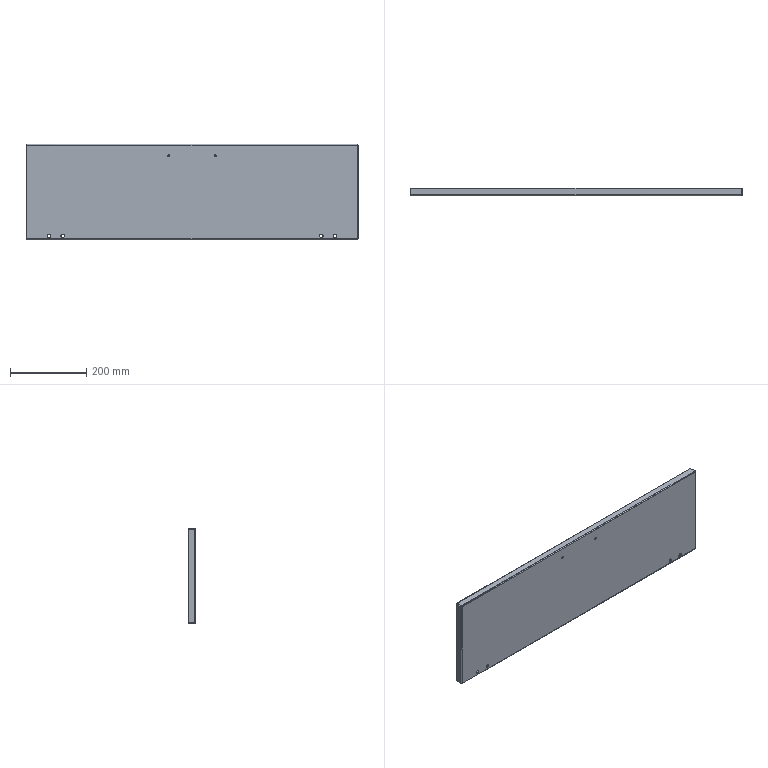Part | SolidWorks | features BaseBody 1 | 1 solid | 54 faces | box 870 x 20 x 250 mm | volume 408515 mm3 | plane 24 | cylinder 22 | spline 8 | commonest cylinder face diameters 9 x8 1.473 x5 4.473 x5 5 x4